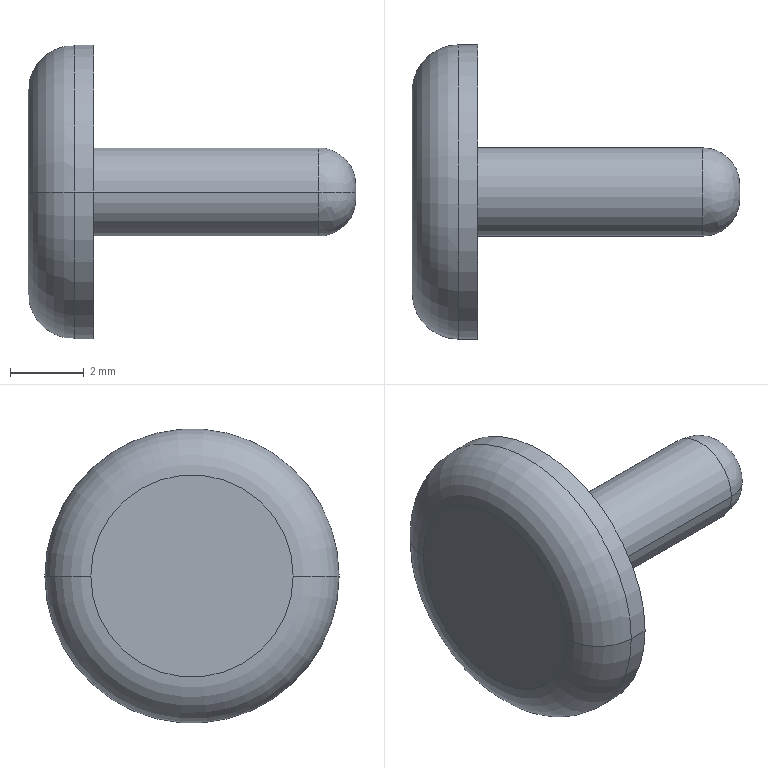Part | STEP file | SR_4060B_1 | 1 solid | 14 faces | box 8.9 x 8 x 8 mm | volume 92.138 mm3 | plane 4 | cylinder 4 | spline 2 | cone 2 | torus 2 | commonest cylinder face diameters 2.4 x2 8 x2
STEP:
#1=CARTESIAN_POINT('',(0.,0.,0.));
#2=DIRECTION('',(0.,0.,1.));
#3=DIRECTION('',(1.,0.,0.));
#4=AXIS2_PLACEMENT_3D('',#1,#2,#3);
#5=CARTESIAN_POINT('',(8.9,0.2,0.));
#6=VERTEX_POINT('',#5);
#7=CARTESIAN_POINT('',(8.9,-0.2,0.));
#8=VERTEX_POINT('',#7);
#9=CARTESIAN_POINT('',(8.9,0.,0.));
#10=DIRECTION('',(-1.,0.,0.));
#11=DIRECTION('',(0.,1.,0.));
#12=AXIS2_PLACEMENT_3D('',#9,#10,#11);
#13=CIRCLE('',#12,0.2);
#14=CARTESIAN_POINT('',(8.9,0.,0.));
#15=DIRECTION('',(1.,0.,0.));
#16=DIRECTION('',(0.,-1.,0.));
#17=AXIS2_PLACEMENT_3D('',#14,#15,#16);
#18=PLANE('',#17);
#19=CARTESIAN_POINT('',(-0.2,0.));
#20=CARTESIAN_POINT('',(-0.2,0.3464));
#21=CARTESIAN_POINT('',(0.1,0.1732));
#22=CARTESIAN_POINT('',(0.4,0.));
#23=CARTESIAN_POINT('',(0.1,-0.1732));
#24=CARTESIAN_POINT('',(-0.2,-0.3464));
#25=CARTESIAN_POINT('',(-0.2,0.));
#26=(BOUNDED_CURVE()B_SPLINE_CURVE(2,(#19,#20,#21,#22,#23,#24,#25),.UNSPECIFIED.,.T.,.F.)B_SPLINE_CURVE_WITH_KNOTS((1,2,2,2,2,1),(-2.094,0.,2.094,4.189,6.283,8.378),.UNSPECIFIED.)CURVE()GEOMETRIC_REPRESENTATION_ITEM()RATIONAL_B_SPLINE_CURVE((1.,0.5,1.,0.5,1.,0.5,1.))REPRESENTATION_ITEM(''));
#27=(GEOMETRIC_REPRESENTATION_CONTEXT(2)PARAMETRIC_REPRESENTATION_CONTEXT()REPRESENTATION_CONTEXT('',''));
#28=DEFINITIONAL_REPRESENTATION('',(#26),#27);
#29=PCURVE('',#18,#28);
#30=CARTESIAN_POINT('',(7.869,-1.195,0.1035));
#31=CARTESIAN_POINT('',(8.484,-1.214,0.1052));
#32=CARTESIAN_POINT('',(8.919,-0.7808,0.06762));
#33=CARTESIAN_POINT('',(8.9,-0.168,0.01455));
#34=CARTESIAN_POINT('',(7.869,-1.26,-0.6455));
#35=CARTESIAN_POINT('',(8.484,-1.28,-0.6559));
#36=CARTESIAN_POINT('',(8.919,-0.8231,-0.4217));
#37=CARTESIAN_POINT('',(8.9,-0.1771,-0.09072));
#38=CARTESIAN_POINT('',(7.869,-0.7518,-1.2));
#39=CARTESIAN_POINT('',(8.484,-0.7639,-1.219));
#40=CARTESIAN_POINT('',(8.919,-0.4912,-0.7837));
#41=CARTESIAN_POINT('',(8.9,-0.1057,-0.1686));
#42=CARTESIAN_POINT('',(7.869,0.,-1.2));
#43=CARTESIAN_POINT('',(8.484,0.,-1.219));
#44=CARTESIAN_POINT('',(8.919,0.,-0.7837));
#45=CARTESIAN_POINT('',(8.9,0.,-0.1686));
#46=CARTESIAN_POINT('',(7.869,0.7518,-1.2));
#47=CARTESIAN_POINT('',(8.484,0.7639,-1.219));
#48=CARTESIAN_POINT('',(8.919,0.4912,-0.7837));
#49=CARTESIAN_POINT('',(8.9,0.1057,-0.1686));
#50=CARTESIAN_POINT('',(7.869,1.26,-0.6455));
#51=CARTESIAN_POINT('',(8.484,1.28,-0.6559));
#52=CARTESIAN_POINT('',(8.919,0.8231,-0.4217));
#53=CARTESIAN_POINT('',(8.9,0.1771,-0.09072));
#54=CARTESIAN_POINT('',(7.869,1.195,0.1035));
#55=CARTESIAN_POINT('',(8.484,1.214,0.1052));
#56=CARTESIAN_POINT('',(8.919,0.7808,0.06762));
#57=CARTESIAN_POINT('',(8.9,0.168,0.01455));
#58=(BOUNDED_SURFACE()B_SPLINE_SURFACE(3,3,((#30,#31,#32,#33),(#34,#35,#36,#37),(#38,#39,#40,#41),(#42,#43,#44,#45),(#46,#47,#48,#49),(#50,#51,#52,#53),(#54,#55,#56,#57)),.UNSPECIFIED.,.F.,.F.,.F.)B_SPLINE_SURFACE_WITH_KNOTS((4,3,4),(4,4),(0.,1.,2.),(0.,1.),.PIECEWISE_BEZIER_KNOTS.)GEOMETRIC_REPRESENTATION_ITEM()RATIONAL_B_SPLINE_SURFACE(((1.417,1.119,1.119,1.417),(1.111,0.8771,0.8771,1.111),(1.111,0.8771,0.8771,1.111),(1.417,1.119,1.119,1.417),(1.111,0.8771,0.8771,1.111),(1.111,0.8771,0.8771,1.111),(1.417,1.119,1.119,1.417)))REPRESENTATION_ITEM('')SURFACE());
#59=CARTESIAN_POINT('',(1.942,0.9786));
#60=CARTESIAN_POINT('',(1.911,0.9786));
#61=CARTESIAN_POINT('',(1.851,0.9786));
#62=CARTESIAN_POINT('',(1.764,0.9786));
#63=CARTESIAN_POINT('',(1.68,0.9786));
#64=CARTESIAN_POINT('',(1.597,0.9786));
#65=CARTESIAN_POINT('',(1.516,0.9786));
#66=CARTESIAN_POINT('',(1.435,0.9786));
#67=CARTESIAN_POINT('',(1.353,0.9786));
#68=CARTESIAN_POINT('',(1.27,0.9786));
#69=CARTESIAN_POINT('',(1.184,0.9786));
#70=CARTESIAN_POINT('',(1.095,0.9786));
#71=CARTESIAN_POINT('',(1.,0.9786));
#72=CARTESIAN_POINT('',(0.9049,0.9786));
#73=CARTESIAN_POINT('',(0.816,0.9786));
#74=CARTESIAN_POINT('',(0.7302,0.9786));
#75=CARTESIAN_POINT('',(0.6469,0.9786));
#76=CARTESIAN_POINT('',(0.5651,0.9786));
#77=CARTESIAN_POINT('',(0.484,0.9786));
#78=CARTESIAN_POINT('',(0.4027,0.9786));
#79=CARTESIAN_POINT('',(0.3204,0.9786));
#80=CARTESIAN_POINT('',(0.2363,0.9786));
#81=CARTESIAN_POINT('',(0.1493,0.9786));
#82=CARTESIAN_POINT('',(0.0887,0.9786));
#83=CARTESIAN_POINT('',(0.05755,0.9786));
#84=B_SPLINE_CURVE_WITH_KNOTS('',3,(#59,#60,#61,#62,#63,#64,#65,#66,#67,#68,#69,#70,#71,#72,#73,#74,#75,#76,#77,#78,#79,#80,#81,#82,#83),.UNSPECIFIED.,.F.,.F.,(4,1,1,1,1,1,1,1,1,1,1,1,1,1,1,1,1,1,1,1,1,1,4),(0.,0.1428,0.2856,0.4284,0.5712,0.714,0.8568,0.9996,1.142,1.285,1.428,1.571,1.714,1.856,1.999,2.142,2.285,2.428,2.57,2.713,2.856,2.999,3.142),.QUASI_UNIFORM_KNOTS.);
#85=(GEOMETRIC_REPRESENTATION_CONTEXT(2)PARAMETRIC_REPRESENTATION_CONTEXT()REPRESENTATION_CONTEXT('',''));
#86=DEFINITIONAL_REPRESENTATION('',(#84),#85);
#87=PCURVE('',#58,#86);
#88=SURFACE_CURVE('',#13,(#29,#87),.PCURVE_S1.);
#89=EDGE_CURVE('',#6,#8,#88,.T.);
#90=ORIENTED_EDGE('',*,*,#89,.T.);
#91=CARTESIAN_POINT('',(8.9,0.,0.));
#92=DIRECTION('',(1.,0.,0.));
#93=DIRECTION('',(0.,1.,0.));
#94=AXIS2_PLACEMENT_3D('',#91,#92,#93);
#95=CIRCLE('',#94,0.2);
#96=CARTESIAN_POINT('',(0.,0.));
#97=DIRECTION('',(-1.,0.));
#98=AXIS2_PLACEMENT_2D('',#96,#97);
#99=CIRCLE('',#98,0.2);
#100=(GEOMETRIC_REPRESENTATION_CONTEXT(2)PARAMETRIC_REPRESENTATION_CONTEXT()REPRESENTATION_CONTEXT('',''));
#101=DEFINITIONAL_REPRESENTATION('',(#99),#100);
#102=PCURVE('',#18,#101);
#103=CARTESIAN_POINT('',(7.869,1.195,-0.1035));
#104=CARTESIAN_POINT('',(8.484,1.214,-0.1052));
#105=CARTESIAN_POINT('',(8.919,0.7808,-0.06762));
#106=CARTESIAN_POINT('',(8.9,0.168,-0.01455));
#107=CARTESIAN_POINT('',(7.869,1.26,0.6455));
#108=CARTESIAN_POINT('',(8.484,1.28,0.6559));
#109=CARTESIAN_POINT('',(8.919,0.8231,0.4217));
#110=CARTESIAN_POINT('',(8.9,0.1771,0.09072));
#111=CARTESIAN_POINT('',(7.869,0.7518,1.2));
#112=CARTESIAN_POINT('',(8.484,0.7639,1.219));
#113=CARTESIAN_POINT('',(8.919,0.4912,0.7837));
#114=CARTESIAN_POINT('',(8.9,0.1057,0.1686));
#115=CARTESIAN_POINT('',(7.869,0.,1.2));
#116=CARTESIAN_POINT('',(8.484,0.,1.219));
#117=CARTESIAN_POINT('',(8.919,0.,0.7837));
#118=CARTESIAN_POINT('',(8.9,0.,0.1686));
#119=CARTESIAN_POINT('',(7.869,-0.7518,1.2));
#120=CARTESIAN_POINT('',(8.484,-0.7639,1.219));
#121=CARTESIAN_POINT('',(8.919,-0.4912,0.7837));
#122=CARTESIAN_POINT('',(8.9,-0.1057,0.1686));
#123=CARTESIAN_POINT('',(7.869,-1.26,0.6455));
#124=CARTESIAN_POINT('',(8.484,-1.28,0.6559));
#125=CARTESIAN_POINT('',(8.919,-0.8231,0.4217));
#126=CARTESIAN_POINT('',(8.9,-0.1771,0.09072));
#127=CARTESIAN_POINT('',(7.869,-1.195,-0.1035));
#128=CARTESIAN_POINT('',(8.484,-1.214,-0.1052));
#129=CARTESIAN_POINT('',(8.919,-0.7808,-0.06762));
#130=CARTESIAN_POINT('',(8.9,-0.168,-0.01455));
#131=(BOUNDED_SURFACE()B_SPLINE_SURFACE(3,3,((#103,#104,#105,#106),(#107,#108,#109,#110),(#111,#112,#113,#114),(#115,#116,#117,#118),(#119,#120,#121,#122),(#123,#124,#125,#126),(#127,#128,#129,#130)),.UNSPECIFIED.,.F.,.F.,.F.)B_SPLINE_SURFACE_WITH_KNOTS((4,3,4),(4,4),(0.,1.,2.),(0.,1.),.PIECEWISE_BEZIER_KNOTS.)GEOMETRIC_REPRESENTATION_ITEM()RATIONAL_B_SPLINE_SURFACE(((1.417,1.119,1.119,1.417),(1.111,0.8771,0.8771,1.111),(1.111,0.8771,0.8771,1.111),(1.417,1.119,1.119,1.417),(1.111,0.8771,0.8771,1.111),(1.111,0.8771,0.8771,1.111),(1.417,1.119,1.119,1.417)))REPRESENTATION_ITEM('')SURFACE());
#132=CARTESIAN_POINT('',(0.05755,0.9786));
#133=CARTESIAN_POINT('',(0.0887,0.9786));
#134=CARTESIAN_POINT('',(0.1493,0.9786));
#135=CARTESIAN_POINT('',(0.2363,0.9786));
#136=CARTESIAN_POINT('',(0.3204,0.9786));
#137=CARTESIAN_POINT('',(0.4027,0.9786));
#138=CARTESIAN_POINT('',(0.484,0.9786));
#139=CARTESIAN_POINT('',(0.5651,0.9786));
#140=CARTESIAN_POINT('',(0.6469,0.9786));
#141=CARTESIAN_POINT('',(0.7302,0.9786));
#142=CARTESIAN_POINT('',(0.816,0.9786));
#143=CARTESIAN_POINT('',(0.9049,0.9786));
#144=CARTESIAN_POINT('',(1.,0.9786));
#145=CARTESIAN_POINT('',(1.095,0.9786));
#146=CARTESIAN_POINT('',(1.184,0.9786));
#147=CARTESIAN_POINT('',(1.27,0.9786));
#148=CARTESIAN_POINT('',(1.353,0.9786));
#149=CARTESIAN_POINT('',(1.435,0.9786));
#150=CARTESIAN_POINT('',(1.516,0.9786));
#151=CARTESIAN_POINT('',(1.597,0.9786));
#152=CARTESIAN_POINT('',(1.68,0.9786));
#153=CARTESIAN_POINT('',(1.764,0.9786));
#154=CARTESIAN_POINT('',(1.851,0.9786));
#155=CARTESIAN_POINT('',(1.911,0.9786));
#156=CARTESIAN_POINT('',(1.942,0.9786));
#157=B_SPLINE_CURVE_WITH_KNOTS('',3,(#132,#133,#134,#135,#136,#137,#138,#139,#140,#141,#142,#143,#144,#145,#146,#147,#148,#149,#150,#151,#152,#153,#154,#155,#156),.UNSPECIFIED.,.F.,.F.,(4,1,1,1,1,1,1,1,1,1,1,1,1,1,1,1,1,1,1,1,1,1,4),(0.,0.1428,0.2856,0.4284,0.5712,0.714,0.8568,0.9996,1.142,1.285,1.428,1.571,1.714,1.856,1.999,2.142,2.285,2.428,2.57,2.713,2.856,2.999,3.142),.QUASI_UNIFORM_KNOTS.);
#158=(GEOMETRIC_REPRESENTATION_CONTEXT(2)PARAMETRIC_REPRESENTATION_CONTEXT()REPRESENTATION_CONTEXT('',''));
#159=DEFINITIONAL_REPRESENTATION('',(#157),#158);
#160=PCURVE('',#131,#159);
#161=SURFACE_CURVE('',#95,(#102,#160),.PCURVE_S1.);
#162=EDGE_CURVE('',#6,#8,#161,.T.);
#163=ORIENTED_EDGE('',*,*,#162,.F.);
#164=EDGE_LOOP('',(#90,#163));
#165=FACE_BOUND('',#164,.F.);
#166=ADVANCED_FACE('',(#165),#18,.T.);
#167=ORIENTED_EDGE('',*,*,#89,.T.);
#168=CARTESIAN_POINT('',(7.9,-1.2,0.));
#169=VERTEX_POINT('',#168);
#170=CARTESIAN_POINT('',(7.9,-0.2,0.));
#171=DIRECTION('',(0.,0.,-1.));
#172=DIRECTION('',(1.,0.,0.));
#173=AXIS2_PLACEMENT_3D('',#170,#171,#172);
#174=CIRCLE('',#173,1.);
#175=CARTESIAN_POINT('',(0.05755,0.9786));
#176=CARTESIAN_POINT('',(0.05755,0.9625));
#177=CARTESIAN_POINT('',(0.05755,0.9307));
#178=CARTESIAN_POINT('',(0.05755,0.8844));
#179=CARTESIAN_POINT('',(0.05755,0.8391));
#180=CARTESIAN_POINT('',(0.05755,0.7948));
#181=CARTESIAN_POINT('',(0.05755,0.7512));
#182=CARTESIAN_POINT('',(0.05755,0.7084));
#183=CARTESIAN_POINT('',(0.05755,0.6661));
#184=CARTESIAN_POINT('',(0.05755,0.6242));
#185=CARTESIAN_POINT('',(0.05755,0.5826));
#186=CARTESIAN_POINT('',(0.05755,0.5412));
#187=CARTESIAN_POINT('',(0.05755,0.5));
#188=CARTESIAN_POINT('',(0.05755,0.4588));
#189=CARTESIAN_POINT('',(0.05755,0.4174));
#190=CARTESIAN_POINT('',(0.05755,0.3758));
#191=CARTESIAN_POINT('',(0.05755,0.3339));
#192=CARTESIAN_POINT('',(0.05755,0.2916));
#193=CARTESIAN_POINT('',(0.05755,0.2488));
#194=CARTESIAN_POINT('',(0.05755,0.2052));
#195=CARTESIAN_POINT('',(0.05755,0.1609));
#196=CARTESIAN_POINT('',(0.05755,0.1156));
#197=CARTESIAN_POINT('',(0.05755,0.06926));
#198=CARTESIAN_POINT('',(0.05755,0.03751));
#199=CARTESIAN_POINT('',(0.05755,0.0214));
#200=B_SPLINE_CURVE_WITH_KNOTS('',3,(#175,#176,#177,#178,#179,#180,#181,#182,#183,#184,#185,#186,#187,#188,#189,#190,#191,#192,#193,#194,#195,#196,#197,#198,#199),.UNSPECIFIED.,.F.,.F.,(4,1,1,1,1,1,1,1,1,1,1,1,1,1,1,1,1,1,1,1,1,1,4),(0.,0.0714,0.1428,0.2142,0.2856,0.357,0.4284,0.4998,0.5712,0.6426,0.714,0.7854,0.8568,0.9282,0.9996,1.071,1.142,1.214,1.285,1.357,1.428,1.499,1.571),.QUASI_UNIFORM_KNOTS.);
#201=(GEOMETRIC_REPRESENTATION_CONTEXT(2)PARAMETRIC_REPRESENTATION_CONTEXT()REPRESENTATION_CONTEXT('',''));
#202=DEFINITIONAL_REPRESENTATION('',(#200),#201);
#203=PCURVE('',#58,#202);
#204=CARTESIAN_POINT('',(1.942,0.9786));
#205=CARTESIAN_POINT('',(1.942,0.9625));
#206=CARTESIAN_POINT('',(1.942,0.9307));
#207=CARTESIAN_POINT('',(1.942,0.8844));
#208=CARTESIAN_POINT('',(1.942,0.8391));
#209=CARTESIAN_POINT('',(1.942,0.7948));
#210=CARTESIAN_POINT('',(1.942,0.7512));
#211=CARTESIAN_POINT('',(1.942,0.7084));
#212=CARTESIAN_POINT('',(1.942,0.6661));
#213=CARTESIAN_POINT('',(1.942,0.6242));
#214=CARTESIAN_POINT('',(1.942,0.5826));
#215=CARTESIAN_POINT('',(1.942,0.5412));
#216=CARTESIAN_POINT('',(1.942,0.5));
#217=CARTESIAN_POINT('',(1.942,0.4588));
#218=CARTESIAN_POINT('',(1.942,0.4174));
#219=CARTESIAN_POINT('',(1.942,0.3758));
#220=CARTESIAN_POINT('',(1.942,0.3339));
#221=CARTESIAN_POINT('',(1.942,0.2916));
#222=CARTESIAN_POINT('',(1.942,0.2488));
#223=CARTESIAN_POINT('',(1.942,0.2052));
#224=CARTESIAN_POINT('',(1.942,0.1609));
#225=CARTESIAN_POINT('',(1.942,0.1156));
#226=CARTESIAN_POINT('',(1.942,0.06926));
#227=CARTESIAN_POINT('',(1.942,0.03751));
#228=CARTESIAN_POINT('',(1.942,0.0214));
#229=B_SPLINE_CURVE_WITH_KNOTS('',3,(#204,#205,#206,#207,#208,#209,#210,#211,#212,#213,#214,#215,#216,#217,#218,#219,#220,#221,#222,#223,#224,#225,#226,#227,#228),.UNSPECIFIED.,.F.,.F.,(4,1,1,1,1,1,1,1,1,1,1,1,1,1,1,1,1,1,1,1,1,1,4),(0.,0.0714,0.1428,0.2142,0.2856,0.357,0.4284,0.4998,0.5712,0.6426,0.714,0.7854,0.8568,0.9282,0.9996,1.071,1.142,1.214,1.285,1.357,1.428,1.499,1.571),.QUASI_UNIFORM_KNOTS.);
#230=(GEOMETRIC_REPRESENTATION_CONTEXT(2)PARAMETRIC_REPRESENTATION_CONTEXT()REPRESENTATION_CONTEXT('',''));
#231=DEFINITIONAL_REPRESENTATION('',(#229),#230);
#232=PCURVE('',#131,#231);
#233=SURFACE_CURVE('',#174,(#203,#232),.PCURVE_S1.);
#234=EDGE_CURVE('',#8,#169,#233,.T.);
#235=ORIENTED_EDGE('',*,*,#234,.T.);
#236=CARTESIAN_POINT('',(7.9,1.2,0.));
#237=VERTEX_POINT('',#236);
#238=CARTESIAN_POINT('',(7.9,0.,0.));
#239=DIRECTION('',(-1.,0.,0.));
#240=DIRECTION('',(0.,1.,0.));
#241=AXIS2_PLACEMENT_3D('',#238,#239,#240);
#242=CIRCLE('',#241,1.2);
#243=CARTESIAN_POINT('',(1.942,0.0214));
#244=CARTESIAN_POINT('',(1.911,0.0214));
#245=CARTESIAN_POINT('',(1.851,0.0214));
#246=CARTESIAN_POINT('',(1.764,0.0214));
#247=CARTESIAN_POINT('',(1.68,0.0214));
#248=CARTESIAN_POINT('',(1.597,0.0214));
#249=CARTESIAN_POINT('',(1.516,0.0214));
#250=CARTESIAN_POINT('',(1.435,0.0214));
#251=CARTESIAN_POINT('',(1.353,0.0214));
#252=CARTESIAN_POINT('',(1.27,0.0214));
#253=CARTESIAN_POINT('',(1.184,0.0214));
#254=CARTESIAN_POINT('',(1.095,0.0214));
#255=CARTESIAN_POINT('',(1.,0.0214));
#256=CARTESIAN_POINT('',(0.9049,0.0214));
#257=CARTESIAN_POINT('',(0.816,0.0214));
#258=CARTESIAN_POINT('',(0.7302,0.0214));
#259=CARTESIAN_POINT('',(0.6469,0.0214));
#260=CARTESIAN_POINT('',(0.5651,0.0214));
#261=CARTESIAN_POINT('',(0.484,0.0214));
#262=CARTESIAN_POINT('',(0.4027,0.0214));
#263=CARTESIAN_POINT('',(0.3204,0.0214));
#264=CARTESIAN_POINT('',(0.2363,0.0214));
#265=CARTESIAN_POINT('',(0.1493,0.0214));
#266=CARTESIAN_POINT('',(0.0887,0.0214));
#267=CARTESIAN_POINT('',(0.05755,0.0214));
#268=B_SPLINE_CURVE_WITH_KNOTS('',3,(#243,#244,#245,#246,#247,#248,#249,#250,#251,#252,#253,#254,#255,#256,#257,#258,#259,#260,#261,#262,#263,#264,#265,#266,#267),.UNSPECIFIED.,.F.,.F.,(4,1,1,1,1,1,1,1,1,1,1,1,1,1,1,1,1,1,1,1,1,1,4),(0.,0.1428,0.2856,0.4284,0.5712,0.714,0.8568,0.9996,1.142,1.285,1.428,1.571,1.714,1.856,1.999,2.142,2.285,2.428,2.57,2.713,2.856,2.999,3.142),.QUASI_UNIFORM_KNOTS.);
#269=(GEOMETRIC_REPRESENTATION_CONTEXT(2)PARAMETRIC_REPRESENTATION_CONTEXT()REPRESENTATION_CONTEXT('',''));
#270=DEFINITIONAL_REPRESENTATION('',(#268),#269);
#271=PCURVE('',#58,#270);
#272=CARTESIAN_POINT('',(-0.445,0.,0.));
#273=DIRECTION('',(1.,0.,0.));
#274=DIRECTION('',(0.,-1.,0.));
#275=AXIS2_PLACEMENT_3D('',#272,#273,#274);
#276=CYLINDRICAL_SURFACE('',#275,1.2);
#277=CARTESIAN_POINT('',(3.142,8.345));
#278=DIRECTION('',(-1.,0.));
#279=VECTOR('',#278,1.);
#280=LINE('',#277,#279);
#281=(GEOMETRIC_REPRESENTATION_CONTEXT(2)PARAMETRIC_REPRESENTATION_CONTEXT()REPRESENTATION_CONTEXT('',''));
#282=DEFINITIONAL_REPRESENTATION('',(#280),#281);
#283=PCURVE('',#276,#282);
#284=SURFACE_CURVE('',#242,(#271,#283),.PCURVE_S1.);
#285=EDGE_CURVE('',#237,#169,#284,.T.);
#286=ORIENTED_EDGE('',*,*,#285,.F.);
#287=CARTESIAN_POINT('',(7.9,0.2,0.));
#288=DIRECTION('',(0.,0.,1.));
#289=DIRECTION('',(1.,0.,0.));
#290=AXIS2_PLACEMENT_3D('',#287,#288,#289);
#291=CIRCLE('',#290,1.);
#292=CARTESIAN_POINT('',(1.942,0.9786));
#293=CARTESIAN_POINT('',(1.942,0.9625));
#294=CARTESIAN_POINT('',(1.942,0.9307));
#295=CARTESIAN_POINT('',(1.942,0.8844));
#296=CARTESIAN_POINT('',(1.942,0.8391));
#297=CARTESIAN_POINT('',(1.942,0.7948));
#298=CARTESIAN_POINT('',(1.942,0.7512));
#299=CARTESIAN_POINT('',(1.942,0.7084));
#300=CARTESIAN_POINT('',(1.942,0.6661));
#301=CARTESIAN_POINT('',(1.942,0.6242));
#302=CARTESIAN_POINT('',(1.942,0.5826));
#303=CARTESIAN_POINT('',(1.942,0.5412));
#304=CARTESIAN_POINT('',(1.942,0.5));
#305=CARTESIAN_POINT('',(1.942,0.4588));
#306=CARTESIAN_POINT('',(1.942,0.4174));
#307=CARTESIAN_POINT('',(1.942,0.3758));
#308=CARTESIAN_POINT('',(1.942,0.3339));
#309=CARTESIAN_POINT('',(1.942,0.2916));
#310=CARTESIAN_POINT('',(1.942,0.2488));
#311=CARTESIAN_POINT('',(1.942,0.2052));
#312=CARTESIAN_POINT('',(1.942,0.1609));
#313=CARTESIAN_POINT('',(1.942,0.1156));
#314=CARTESIAN_POINT('',(1.942,0.06926));
#315=CARTESIAN_POINT('',(1.942,0.03751));
#316=CARTESIAN_POINT('',(1.942,0.0214));
#317=B_SPLINE_CURVE_WITH_KNOTS('',3,(#292,#293,#294,#295,#296,#297,#298,#299,#300,#301,#302,#303,#304,#305,#306,#307,#308,#309,#310,#311,#312,#313,#314,#315,#316),.UNSPECIFIED.,.F.,.F.,(4,1,1,1,1,1,1,1,1,1,1,1,1,1,1,1,1,1,1,1,1,1,4),(0.,0.0714,0.1428,0.2142,0.2856,0.357,0.4284,0.4998,0.5712,0.6426,0.714,0.7854,0.8568,0.9282,0.9996,1.071,1.142,1.214,1.285,1.357,1.428,1.499,1.571),.QUASI_UNIFORM_KNOTS.);
#318=(GEOMETRIC_REPRESENTATION_CONTEXT(2)PARAMETRIC_REPRESENTATION_CONTEXT()REPRESENTATION_CONTEXT('',''));
#319=DEFINITIONAL_REPRESENTATION('',(#317),#318);
#320=PCURVE('',#58,#319);
#321=CARTESIAN_POINT('',(0.05755,0.9786));
#322=CARTESIAN_POINT('',(0.05755,0.9625));
#323=CARTESIAN_POINT('',(0.05755,0.9307));
#324=CARTESIAN_POINT('',(0.05755,0.8844));
#325=CARTESIAN_POINT('',(0.05755,0.8391));
#326=CARTESIAN_POINT('',(0.05755,0.7948));
#327=CARTESIAN_POINT('',(0.05755,0.7512));
#328=CARTESIAN_POINT('',(0.05755,0.7084));
#329=CARTESIAN_POINT('',(0.05755,0.6661));
#330=CARTESIAN_POINT('',(0.05755,0.6242));
#331=CARTESIAN_POINT('',(0.05755,0.5826));
#332=CARTESIAN_POINT('',(0.05755,0.5412));
#333=CARTESIAN_POINT('',(0.05755,0.5));
#334=CARTESIAN_POINT('',(0.05755,0.4588));
#335=CARTESIAN_POINT('',(0.05755,0.4174));
#336=CARTESIAN_POINT('',(0.05755,0.3758));
#337=CARTESIAN_POINT('',(0.05755,0.3339));
#338=CARTESIAN_POINT('',(0.05755,0.2916));
#339=CARTESIAN_POINT('',(0.05755,0.2488));
#340=CARTESIAN_POINT('',(0.05755,0.2052));
#341=CARTESIAN_POINT('',(0.05755,0.1609));
#342=CARTESIAN_POINT('',(0.05755,0.1156));
#343=CARTESIAN_POINT('',(0.05755,0.06926));
#344=CARTESIAN_POINT('',(0.05755,0.03751));
#345=CARTESIAN_POINT('',(0.05755,0.0214));
#346=B_SPLINE_CURVE_WITH_KNOTS('',3,(#321,#322,#323,#324,#325,#326,#327,#328,#329,#330,#331,#332,#333,#334,#335,#336,#337,#338,#339,#340,#341,#342,#343,#344,#345),.UNSPECIFIED.,.F.,.F.,(4,1,1,1,1,1,1,1,1,1,1,1,1,1,1,1,1,1,1,1,1,1,4),(0.,0.0714,0.1428,0.2142,0.2856,0.357,0.4284,0.4998,0.5712,0.6426,0.714,0.7854,0.8568,0.9282,0.9996,1.071,1.142,1.214,1.285,1.357,1.428,1.499,1.571),.QUASI_UNIFORM_KNOTS.);
#347=(GEOMETRIC_REPRESENTATION_CONTEXT(2)PARAMETRIC_REPRESENTATION_CONTEXT()REPRESENTATION_CONTEXT('',''));
#348=DEFINITIONAL_REPRESENTATION('',(#346),#347);
#349=PCURVE('',#131,#348);
#350=SURFACE_CURVE('',#291,(#320,#349),.PCURVE_S1.);
#351=EDGE_CURVE('',#6,#237,#350,.T.);
#352=ORIENTED_EDGE('',*,*,#351,.F.);
#353=EDGE_LOOP('',(#167,#235,#286,#352));
#354=FACE_BOUND('',#353,.T.);
#355=ADVANCED_FACE('',(#354),#58,.T.);
#356=CARTESIAN_POINT('',(7.9,0.,0.));
#357=DIRECTION('',(1.,0.,0.));
#358=DIRECTION('',(0.,1.,0.));
#359=AXIS2_PLACEMENT_3D('',#356,#357,#358);
#360=CIRCLE('',#359,1.2);
#361=CARTESIAN_POINT('',(0.05755,0.0214));
#362=CARTESIAN_POINT('',(0.0887,0.0214));
#363=CARTESIAN_POINT('',(0.1493,0.0214));
#364=CARTESIAN_POINT('',(0.2363,0.0214));
#365=CARTESIAN_POINT('',(0.3204,0.0214));
#366=CARTESIAN_POINT('',(0.4027,0.0214));
#367=CARTESIAN_POINT('',(0.484,0.0214));
#368=CARTESIAN_POINT('',(0.5651,0.0214));
#369=CARTESIAN_POINT('',(0.6469,0.0214));
#370=CARTESIAN_POINT('',(0.7302,0.0214));
#371=CARTESIAN_POINT('',(0.816,0.0214));
#372=CARTESIAN_POINT('',(0.9049,0.0214));
#373=CARTESIAN_POINT('',(1.,0.0214));
#374=CARTESIAN_POINT('',(1.095,0.0214));
#375=CARTESIAN_POINT('',(1.184,0.0214));
#376=CARTESIAN_POINT('',(1.27,0.0214));
#377=CARTESIAN_POINT('',(1.353,0.0214));
#378=CARTESIAN_POINT('',(1.435,0.0214));
#379=CARTESIAN_POINT('',(1.516,0.0214));
#380=CARTESIAN_POINT('',(1.597,0.0214));
#381=CARTESIAN_POINT('',(1.68,0.0214));
#382=CARTESIAN_POINT('',(1.764,0.0214));
#383=CARTESIAN_POINT('',(1.851,0.0214));
#384=CARTESIAN_POINT('',(1.911,0.0214));
#385=CARTESIAN_POINT('',(1.942,0.0214));
#386=B_SPLINE_CURVE_WITH_KNOTS('',3,(#361,#362,#363,#364,#365,#366,#367,#368,#369,#370,#371,#372,#373,#374,#375,#376,#377,#378,#379,#380,#381,#382,#383,#384,#385),.UNSPECIFIED.,.F.,.F.,(4,1,1,1,1,1,1,1,1,1,1,1,1,1,1,1,1,1,1,1,1,1,4),(0.,0.1428,0.2856,0.4284,0.5712,0.714,0.8568,0.9996,1.142,1.285,1.428,1.571,1.714,1.856,1.999,2.142,2.285,2.428,2.57,2.713,2.856,2.999,3.142),.QUASI_UNIFORM_KNOTS.);
#387=(GEOMETRIC_REPRESENTATION_CONTEXT(2)PARAMETRIC_REPRESENTATION_CONTEXT()REPRESENTATION_CONTEXT('',''));
#388=DEFINITIONAL_REPRESENTATION('',(#386),#387);
#389=PCURVE('',#131,#388);
#390=CARTESIAN_POINT('',(-0.445,0.,0.));
#391=DIRECTION('',(1.,0.,0.));
#392=DIRECTION('',(0.,-1.,0.));
#393=AXIS2_PLACEMENT_3D('',#390,#391,#392);
#394=CYLINDRICAL_SURFACE('',#393,1.2);
#395=CARTESIAN_POINT('',(3.142,8.345));
#396=DIRECTION('',(1.,0.));
#397=VECTOR('',#396,1.);
#398=LINE('',#395,#397);
#399=(GEOMETRIC_REPRESENTATION_CONTEXT(2)PARAMETRIC_REPRESENTATION_CONTEXT()REPRESENTATION_CONTEXT('',''));
#400=DEFINITIONAL_REPRESENTATION('',(#398),#399);
#401=PCURVE('',#394,#400);
#402=SURFACE_CURVE('',#360,(#389,#401),.PCURVE_S1.);
#403=EDGE_CURVE('',#237,#169,#402,.T.);
#404=ORIENTED_EDGE('',*,*,#403,.T.);
#405=ORIENTED_EDGE('',*,*,#234,.F.);
#406=ORIENTED_EDGE('',*,*,#162,.F.);
#407=ORIENTED_EDGE('',*,*,#351,.T.);
#408=EDGE_LOOP('',(#404,#405,#406,#407));
#409=FACE_BOUND('',#408,.T.);
#410=ADVANCED_FACE('',(#409),#131,.T.);
#411=CARTESIAN_POINT('',(0.9,1.2,0.));
#412=VERTEX_POINT('',#411);
#413=CARTESIAN_POINT('',(0.9,-1.2,0.));
#414=VERTEX_POINT('',#413);
#415=CARTESIAN_POINT('',(0.9,0.,0.));
#416=DIRECTION('',(1.,0.,0.));
#417=DIRECTION('',(0.,1.,0.));
#418=AXIS2_PLACEMENT_3D('',#415,#416,#417);
#419=CIRCLE('',#418,1.2);
#420=CARTESIAN_POINT('',(3.142,1.345));
#421=DIRECTION('',(1.,0.));
#422=VECTOR('',#421,1.);
#423=LINE('',#420,#422);
#424=(GEOMETRIC_REPRESENTATION_CONTEXT(2)PARAMETRIC_REPRESENTATION_CONTEXT()REPRESENTATION_CONTEXT('',''));
#425=DEFINITIONAL_REPRESENTATION('',(#423),#424);
#426=PCURVE('',#394,#425);
#427=CARTESIAN_POINT('',(0.9,0.,0.));
#428=DIRECTION('',(1.,0.,0.));
#429=DIRECTION('',(0.,-1.,0.));
#430=AXIS2_PLACEMENT_3D('',#427,#428,#429);
#431=PLANE('',#430);
#432=CARTESIAN_POINT('',(0.,0.));
#433=DIRECTION('',(-1.,0.));
#434=AXIS2_PLACEMENT_2D('',#432,#433);
#435=CIRCLE('',#434,1.2);
#436=(GEOMETRIC_REPRESENTATION_CONTEXT(2)PARAMETRIC_REPRESENTATION_CONTEXT()REPRESENTATION_CONTEXT('',''));
#437=DEFINITIONAL_REPRESENTATION('',(#435),#436);
#438=PCURVE('',#431,#437);
#439=SURFACE_CURVE('',#419,(#426,#438),.PCURVE_S1.);
#440=EDGE_CURVE('',#412,#414,#439,.T.);
#441=ORIENTED_EDGE('',*,*,#440,.T.);
#442=CARTESIAN_POINT('',(7.9,-1.2,0.));
#443=DIRECTION('',(-1.,0.,0.));
#444=VECTOR('',#443,1.);
#445=LINE('',#442,#444);
#446=CARTESIAN_POINT('',(6.283,8.345));
#447=DIRECTION('',(0.,-1.));
#448=VECTOR('',#447,1.);
#449=LINE('',#446,#448);
#450=(GEOMETRIC_REPRESENTATION_CONTEXT(2)PARAMETRIC_REPRESENTATION_CONTEXT()REPRESENTATION_CONTEXT('',''));
#451=DEFINITIONAL_REPRESENTATION('',(#449),#450);
#452=PCURVE('',#394,#451);
#453=CARTESIAN_POINT('',(0.,8.345));
#454=DIRECTION('',(0.,-1.));
#455=VECTOR('',#454,1.);
#456=LINE('',#453,#455);
#457=(GEOMETRIC_REPRESENTATION_CONTEXT(2)PARAMETRIC_REPRESENTATION_CONTEXT()REPRESENTATION_CONTEXT('',''));
#458=DEFINITIONAL_REPRESENTATION('',(#456),#457);
#459=PCURVE('',#276,#458);
#460=SURFACE_CURVE('',#445,(#452,#459),.PCURVE_S1.);
#461=EDGE_CURVE('',#169,#414,#460,.T.);
#462=ORIENTED_EDGE('',*,*,#461,.F.);
#463=ORIENTED_EDGE('',*,*,#403,.F.);
#464=CARTESIAN_POINT('',(7.9,1.2,0.));
#465=DIRECTION('',(-1.,0.,0.));
#466=VECTOR('',#465,1.);
#467=LINE('',#464,#466);
#468=CARTESIAN_POINT('',(3.142,8.345));
#469=DIRECTION('',(0.,-1.));
#470=VECTOR('',#469,1.);
#471=LINE('',#468,#470);
#472=(GEOMETRIC_REPRESENTATION_CONTEXT(2)PARAMETRIC_REPRESENTATION_CONTEXT()REPRESENTATION_CONTEXT('',''));
#473=DEFINITIONAL_REPRESENTATION('',(#471),#472);
#474=PCURVE('',#394,#473);
#475=CARTESIAN_POINT('',(3.142,8.345));
#476=DIRECTION('',(0.,-1.));
#477=VECTOR('',#476,1.);
#478=LINE('',#475,#477);
#479=(GEOMETRIC_REPRESENTATION_CONTEXT(2)PARAMETRIC_REPRESENTATION_CONTEXT()REPRESENTATION_CONTEXT('',''));
#480=DEFINITIONAL_REPRESENTATION('',(#478),#479);
#481=PCURVE('',#276,#480);
#482=SURFACE_CURVE('',#467,(#474,#481),.PCURVE_S1.);
#483=EDGE_CURVE('',#237,#412,#482,.T.);
#484=ORIENTED_EDGE('',*,*,#483,.T.);
#485=EDGE_LOOP('',(#441,#462,#463,#484));
#486=FACE_BOUND('',#485,.T.);
#487=ADVANCED_FACE('',(#486),#394,.T.);
#488=ORIENTED_EDGE('',*,*,#285,.T.);
#489=ORIENTED_EDGE('',*,*,#461,.T.);
#490=CARTESIAN_POINT('',(0.9,0.,0.));
#491=DIRECTION('',(-1.,0.,0.));
#492=DIRECTION('',(0.,1.,0.));
#493=AXIS2_PLACEMENT_3D('',#490,#491,#492);
#494=CIRCLE('',#493,1.2);
#495=CARTESIAN_POINT('',(3.142,1.345));
#496=DIRECTION('',(-1.,0.));
#497=VECTOR('',#496,1.);
#498=LINE('',#495,#497);
#499=(GEOMETRIC_REPRESENTATION_CONTEXT(2)PARAMETRIC_REPRESENTATION_CONTEXT()REPRESENTATION_CONTEXT('',''));
#500=DEFINITIONAL_REPRESENTATION('',(#498),#499);
#501=PCURVE('',#276,#500);
#502=CARTESIAN_POINT('',(-1.2,0.));
#503=CARTESIAN_POINT('',(-1.2,2.078));
#504=CARTESIAN_POINT('',(0.6,1.039));
#505=CARTESIAN_POINT('',(2.4,0.));
#506=CARTESIAN_POINT('',(0.6,-1.039));
#507=CARTESIAN_POINT('',(-1.2,-2.078));
#508=CARTESIAN_POINT('',(-1.2,0.));
#509=(BOUNDED_CURVE()B_SPLINE_CURVE(2,(#502,#503,#504,#505,#506,#507,#508),.UNSPECIFIED.,.T.,.F.)B_SPLINE_CURVE_WITH_KNOTS((1,2,2,2,2,1),(-2.094,0.,2.094,4.189,6.283,8.378),.UNSPECIFIED.)CURVE()GEOMETRIC_REPRESENTATION_ITEM()RATIONAL_B_SPLINE_CURVE((1.,0.5,1.,0.5,1.,0.5,1.))REPRESENTATION_ITEM(''));
#510=(GEOMETRIC_REPRESENTATION_CONTEXT(2)PARAMETRIC_REPRESENTATION_CONTEXT()REPRESENTATION_CONTEXT('',''));
#511=DEFINITIONAL_REPRESENTATION('',(#509),#510);
#512=PCURVE('',#431,#511);
#513=SURFACE_CURVE('',#494,(#501,#512),.PCURVE_S1.);
#514=EDGE_CURVE('',#412,#414,#513,.T.);
#515=ORIENTED_EDGE('',*,*,#514,.F.);
#516=ORIENTED_EDGE('',*,*,#483,.F.);
#517=EDGE_LOOP('',(#488,#489,#515,#516));
#518=FACE_BOUND('',#517,.T.);
#519=ADVANCED_FACE('',(#518),#276,.T.);
#520=CARTESIAN_POINT('',(0.9,2.7,0.));
#521=VERTEX_POINT('',#520);
#522=CARTESIAN_POINT('',(0.9,-2.7,0.));
#523=VERTEX_POINT('',#522);
#524=CARTESIAN_POINT('',(0.9,0.,0.));
#525=DIRECTION('',(-1.,0.,0.));
#526=DIRECTION('',(0.,1.,0.));
#527=AXIS2_PLACEMENT_3D('',#524,#525,#526);
#528=CIRCLE('',#527,2.7);
#529=CARTESIAN_POINT('',(-2.7,0.));
#530=CARTESIAN_POINT('',(-2.7,4.677));
#531=CARTESIAN_POINT('',(1.35,2.338));
#532=CARTESIAN_POINT('',(5.4,0.));
#533=CARTESIAN_POINT('',(1.35,-2.338));
#534=CARTESIAN_POINT('',(-2.7,-4.677));
#535=CARTESIAN_POINT('',(-2.7,0.));
#536=(BOUNDED_CURVE()B_SPLINE_CURVE(2,(#529,#530,#531,#532,#533,#534,#535),.UNSPECIFIED.,.T.,.F.)B_SPLINE_CURVE_WITH_KNOTS((1,2,2,2,2,1),(-2.094,0.,2.094,4.189,6.283,8.378),.UNSPECIFIED.)CURVE()GEOMETRIC_REPRESENTATION_ITEM()RATIONAL_B_SPLINE_CURVE((1.,0.5,1.,0.5,1.,0.5,1.))REPRESENTATION_ITEM(''));
#537=(GEOMETRIC_REPRESENTATION_CONTEXT(2)PARAMETRIC_REPRESENTATION_CONTEXT()REPRESENTATION_CONTEXT('',''));
#538=DEFINITIONAL_REPRESENTATION('',(#536),#537);
#539=PCURVE('',#431,#538);
#540=CARTESIAN_POINT('',(1.34,0.,0.));
#541=DIRECTION('',(1.,0.,0.));
#542=DIRECTION('',(0.,-1.,0.));
#543=AXIS2_PLACEMENT_3D('',#540,#541,#542);
#544=CONICAL_SURFACE('',#543,2.965,0.5421);
#545=CARTESIAN_POINT('',(3.142,-0.44));
#546=DIRECTION('',(-1.,0.));
#547=VECTOR('',#546,1.);
#548=LINE('',#545,#547);
#549=(GEOMETRIC_REPRESENTATION_CONTEXT(2)PARAMETRIC_REPRESENTATION_CONTEXT()REPRESENTATION_CONTEXT('',''));
#550=DEFINITIONAL_REPRESENTATION('',(#548),#549);
#551=PCURVE('',#544,#550);
#552=SURFACE_CURVE('',#528,(#539,#551),.PCURVE_S1.);
#553=EDGE_CURVE('',#521,#523,#552,.T.);
#554=ORIENTED_EDGE('',*,*,#553,.T.);
#555=CARTESIAN_POINT('',(0.9,0.,0.));
#556=DIRECTION('',(1.,0.,0.));
#557=DIRECTION('',(0.,1.,0.));
#558=AXIS2_PLACEMENT_3D('',#555,#556,#557);
#559=CIRCLE('',#558,2.7);
#560=CARTESIAN_POINT('',(0.,0.));
#561=DIRECTION('',(-1.,0.));
#562=AXIS2_PLACEMENT_2D('',#560,#561);
#563=CIRCLE('',#562,2.7);
#564=(GEOMETRIC_REPRESENTATION_CONTEXT(2)PARAMETRIC_REPRESENTATION_CONTEXT()REPRESENTATION_CONTEXT('',''));
#565=DEFINITIONAL_REPRESENTATION('',(#563),#564);
#566=PCURVE('',#431,#565);
#567=CARTESIAN_POINT('',(1.34,0.,0.));
#568=DIRECTION('',(1.,0.,0.));
#569=DIRECTION('',(0.,-1.,0.));
#570=AXIS2_PLACEMENT_3D('',#567,#568,#569);
#571=CONICAL_SURFACE('',#570,2.965,0.5421);
#572=CARTESIAN_POINT('',(3.142,-0.44));
#573=DIRECTION('',(1.,0.));
#574=VECTOR('',#573,1.);
#575=LINE('',#572,#574);
#576=(GEOMETRIC_REPRESENTATION_CONTEXT(2)PARAMETRIC_REPRESENTATION_CONTEXT()REPRESENTATION_CONTEXT('',''));
#577=DEFINITIONAL_REPRESENTATION('',(#575),#576);
#578=PCURVE('',#571,#577);
#579=SURFACE_CURVE('',#559,(#566,#578),.PCURVE_S1.);
#580=EDGE_CURVE('',#521,#523,#579,.T.);
#581=ORIENTED_EDGE('',*,*,#580,.F.);
#582=EDGE_LOOP('',(#554,#581));
#583=FACE_BOUND('',#582,.F.);
#584=ORIENTED_EDGE('',*,*,#440,.T.);
#585=ORIENTED_EDGE('',*,*,#514,.F.);
#586=EDGE_LOOP('',(#584,#585));
#587=FACE_BOUND('',#586,.F.);
#588=ADVANCED_FACE('',(#583,#587),#431,.T.);
#589=CARTESIAN_POINT('',(1.78,3.23,0.));
#590=VERTEX_POINT('',#589);
#591=CARTESIAN_POINT('',(0.9,2.7,0.));
#592=DIRECTION('',(0.8566,0.5159,0.));
#593=VECTOR('',#592,1.);
#594=LINE('',#591,#593);
#595=CARTESIAN_POINT('',(3.142,-0.44));
#596=DIRECTION('',(0.,1.));
#597=VECTOR('',#596,1.);
#598=LINE('',#595,#597);
#599=(GEOMETRIC_REPRESENTATION_CONTEXT(2)PARAMETRIC_REPRESENTATION_CONTEXT()REPRESENTATION_CONTEXT('',''));
#600=DEFINITIONAL_REPRESENTATION('',(#598),#599);
#601=PCURVE('',#544,#600);
#602=CARTESIAN_POINT('',(3.142,-0.44));
#603=DIRECTION('',(0.,1.));
#604=VECTOR('',#603,1.);
#605=LINE('',#602,#604);
#606=(GEOMETRIC_REPRESENTATION_CONTEXT(2)PARAMETRIC_REPRESENTATION_CONTEXT()REPRESENTATION_CONTEXT('',''));
#607=DEFINITIONAL_REPRESENTATION('',(#605),#606);
#608=PCURVE('',#571,#607);
#609=SURFACE_CURVE('',#594,(#601,#608),.PCURVE_S1.);
#610=EDGE_CURVE('',#521,#590,#609,.T.);
#611=ORIENTED_EDGE('',*,*,#610,.T.);
#612=CARTESIAN_POINT('',(1.78,-3.23,0.));
#613=VERTEX_POINT('',#612);
#614=CARTESIAN_POINT('',(1.78,0.,0.));
#615=DIRECTION('',(-1.,0.,0.));
#616=DIRECTION('',(0.,1.,0.));
#617=AXIS2_PLACEMENT_3D('',#614,#615,#616);
#618=CIRCLE('',#617,3.23);
#619=CARTESIAN_POINT('',(3.142,0.44));
#620=DIRECTION('',(-1.,0.));
#621=VECTOR('',#620,1.);
#622=LINE('',#619,#621);
#623=(GEOMETRIC_REPRESENTATION_CONTEXT(2)PARAMETRIC_REPRESENTATION_CONTEXT()REPRESENTATION_CONTEXT('',''));
#624=DEFINITIONAL_REPRESENTATION('',(#622),#623);
#625=PCURVE('',#544,#624);
#626=CARTESIAN_POINT('',(1.78,0.,0.));
#627=DIRECTION('',(1.,0.,0.));
#628=DIRECTION('',(0.,-1.,0.));
#629=AXIS2_PLACEMENT_3D('',#626,#627,#628);
#630=PLANE('',#629);
#631=CARTESIAN_POINT('',(-3.23,0.));
#632=CARTESIAN_POINT('',(-3.23,5.595));
#633=CARTESIAN_POINT('',(1.615,2.797));
#634=CARTESIAN_POINT('',(6.46,0.));
#635=CARTESIAN_POINT('',(1.615,-2.797));
#636=CARTESIAN_POINT('',(-3.23,-5.595));
#637=CARTESIAN_POINT('',(-3.23,0.));
#638=(BOUNDED_CURVE()B_SPLINE_CURVE(2,(#631,#632,#633,#634,#635,#636,#637),.UNSPECIFIED.,.T.,.F.)B_SPLINE_CURVE_WITH_KNOTS((1,2,2,2,2,1),(-2.094,0.,2.094,4.189,6.283,8.378),.UNSPECIFIED.)CURVE()GEOMETRIC_REPRESENTATION_ITEM()RATIONAL_B_SPLINE_CURVE((1.,0.5,1.,0.5,1.,0.5,1.))REPRESENTATION_ITEM(''));
#639=(GEOMETRIC_REPRESENTATION_CONTEXT(2)PARAMETRIC_REPRESENTATION_CONTEXT()REPRESENTATION_CONTEXT('',''));
#640=DEFINITIONAL_REPRESENTATION('',(#638),#639);
#641=PCURVE('',#630,#640);
#642=SURFACE_CURVE('',#618,(#625,#641),.PCURVE_S1.);
#643=EDGE_CURVE('',#590,#613,#642,.T.);
#644=ORIENTED_EDGE('',*,*,#643,.T.);
#645=CARTESIAN_POINT('',(0.9,-2.7,0.));
#646=DIRECTION('',(0.8566,-0.5159,0.));
#647=VECTOR('',#646,1.);
#648=LINE('',#645,#647);
#649=CARTESIAN_POINT('',(0.,-0.44));
#650=DIRECTION('',(0.,1.));
#651=VECTOR('',#650,1.);
#652=LINE('',#649,#651);
#653=(GEOMETRIC_REPRESENTATION_CONTEXT(2)PARAMETRIC_REPRESENTATION_CONTEXT()REPRESENTATION_CONTEXT('',''));
#654=DEFINITIONAL_REPRESENTATION('',(#652),#653);
#655=PCURVE('',#544,#654);
#656=CARTESIAN_POINT('',(6.283,-0.44));
#657=DIRECTION('',(0.,1.));
#658=VECTOR('',#657,1.);
#659=LINE('',#656,#658);
#660=(GEOMETRIC_REPRESENTATION_CONTEXT(2)PARAMETRIC_REPRESENTATION_CONTEXT()REPRESENTATION_CONTEXT('',''));
#661=DEFINITIONAL_REPRESENTATION('',(#659),#660);
#662=PCURVE('',#571,#661);
#663=SURFACE_CURVE('',#648,(#655,#662),.PCURVE_S1.);
#664=EDGE_CURVE('',#523,#613,#663,.T.);
#665=ORIENTED_EDGE('',*,*,#664,.F.);
#666=ORIENTED_EDGE('',*,*,#553,.F.);
#667=EDGE_LOOP('',(#611,#644,#665,#666));
#668=FACE_BOUND('',#667,.F.);
#669=ADVANCED_FACE('',(#668),#544,.F.);
#670=ORIENTED_EDGE('',*,*,#610,.F.);
#671=ORIENTED_EDGE('',*,*,#580,.T.);
#672=ORIENTED_EDGE('',*,*,#664,.T.);
#673=CARTESIAN_POINT('',(1.78,0.,0.));
#674=DIRECTION('',(1.,0.,0.));
#675=DIRECTION('',(0.,1.,0.));
#676=AXIS2_PLACEMENT_3D('',#673,#674,#675);
#677=CIRCLE('',#676,3.23);
#678=CARTESIAN_POINT('',(3.142,0.44));
#679=DIRECTION('',(1.,0.));
#680=VECTOR('',#679,1.);
#681=LINE('',#678,#680);
#682=(GEOMETRIC_REPRESENTATION_CONTEXT(2)PARAMETRIC_REPRESENTATION_CONTEXT()REPRESENTATION_CONTEXT('',''));
#683=DEFINITIONAL_REPRESENTATION('',(#681),#682);
#684=PCURVE('',#571,#683);
#685=CARTESIAN_POINT('',(0.,0.));
#686=DIRECTION('',(-1.,0.));
#687=AXIS2_PLACEMENT_2D('',#685,#686);
#688=CIRCLE('',#687,3.23);
#689=(GEOMETRIC_REPRESENTATION_CONTEXT(2)PARAMETRIC_REPRESENTATION_CONTEXT()REPRESENTATION_CONTEXT('',''));
#690=DEFINITIONAL_REPRESENTATION('',(#688),#689);
#691=PCURVE('',#630,#690);
#692=SURFACE_CURVE('',#677,(#684,#691),.PCURVE_S1.);
#693=EDGE_CURVE('',#590,#613,#692,.T.);
#694=ORIENTED_EDGE('',*,*,#693,.F.);
#695=EDGE_LOOP('',(#670,#671,#672,#694));
#696=FACE_BOUND('',#695,.F.);
#697=ADVANCED_FACE('',(#696),#571,.F.);
#698=CARTESIAN_POINT('',(1.78,4.,0.));
#699=VERTEX_POINT('',#698);
#700=CARTESIAN_POINT('',(1.78,-4.,0.));
#701=VERTEX_POINT('',#700);
#702=CARTESIAN_POINT('',(1.78,0.,0.));
#703=DIRECTION('',(-1.,0.,0.));
#704=DIRECTION('',(0.,1.,0.));
#705=AXIS2_PLACEMENT_3D('',#702,#703,#704);
#706=CIRCLE('',#705,4.);
#707=CARTESIAN_POINT('',(-4.,0.));
#708=CARTESIAN_POINT('',(-4.,6.928));
#709=CARTESIAN_POINT('',(2.,3.464));
#710=CARTESIAN_POINT('',(8.,0.));
#711=CARTESIAN_POINT('',(2.,-3.464));
#712=CARTESIAN_POINT('',(-4.,-6.928));
#713=CARTESIAN_POINT('',(-4.,0.));
#714=(BOUNDED_CURVE()B_SPLINE_CURVE(2,(#707,#708,#709,#710,#711,#712,#713),.UNSPECIFIED.,.T.,.F.)B_SPLINE_CURVE_WITH_KNOTS((1,2,2,2,2,1),(-2.094,0.,2.094,4.189,6.283,8.378),.UNSPECIFIED.)CURVE()GEOMETRIC_REPRESENTATION_ITEM()RATIONAL_B_SPLINE_CURVE((1.,0.5,1.,0.5,1.,0.5,1.))REPRESENTATION_ITEM(''));
#715=(GEOMETRIC_REPRESENTATION_CONTEXT(2)PARAMETRIC_REPRESENTATION_CONTEXT()REPRESENTATION_CONTEXT('',''));
#716=DEFINITIONAL_REPRESENTATION('',(#714),#715);
#717=PCURVE('',#630,#716);
#718=CARTESIAN_POINT('',(-0.445,0.,0.));
#719=DIRECTION('',(1.,0.,0.));
#720=DIRECTION('',(0.,-1.,0.));
#721=AXIS2_PLACEMENT_3D('',#718,#719,#720);
#722=CYLINDRICAL_SURFACE('',#721,4.);
#723=CARTESIAN_POINT('',(3.142,2.225));
#724=DIRECTION('',(-1.,0.));
#725=VECTOR('',#724,1.);
#726=LINE('',#723,#725);
#727=(GEOMETRIC_REPRESENTATION_CONTEXT(2)PARAMETRIC_REPRESENTATION_CONTEXT()REPRESENTATION_CONTEXT('',''));
#728=DEFINITIONAL_REPRESENTATION('',(#726),#727);
#729=PCURVE('',#722,#728);
#730=SURFACE_CURVE('',#706,(#717,#729),.PCURVE_S1.);
#731=EDGE_CURVE('',#699,#701,#730,.T.);
#732=ORIENTED_EDGE('',*,*,#731,.T.);
#733=CARTESIAN_POINT('',(1.78,0.,0.));
#734=DIRECTION('',(1.,0.,0.));
#735=DIRECTION('',(0.,1.,0.));
#736=AXIS2_PLACEMENT_3D('',#733,#734,#735);
#737=CIRCLE('',#736,4.);
#738=CARTESIAN_POINT('',(0.,0.));
#739=DIRECTION('',(-1.,0.));
#740=AXIS2_PLACEMENT_2D('',#738,#739);
#741=CIRCLE('',#740,4.);
#742=(GEOMETRIC_REPRESENTATION_CONTEXT(2)PARAMETRIC_REPRESENTATION_CONTEXT()REPRESENTATION_CONTEXT('',''));
#743=DEFINITIONAL_REPRESENTATION('',(#741),#742);
#744=PCURVE('',#630,#743);
#745=CARTESIAN_POINT('',(-0.445,0.,0.));
#746=DIRECTION('',(1.,0.,0.));
#747=DIRECTION('',(0.,-1.,0.));
#748=AXIS2_PLACEMENT_3D('',#745,#746,#747);
#749=CYLINDRICAL_SURFACE('',#748,4.);
#750=CARTESIAN_POINT('',(3.142,2.225));
#751=DIRECTION('',(1.,0.));
#752=VECTOR('',#751,1.);
#753=LINE('',#750,#752);
#754=(GEOMETRIC_REPRESENTATION_CONTEXT(2)PARAMETRIC_REPRESENTATION_CONTEXT()REPRESENTATION_CONTEXT('',''));
#755=DEFINITIONAL_REPRESENTATION('',(#753),#754);
#756=PCURVE('',#749,#755);
#757=SURFACE_CURVE('',#737,(#744,#756),.PCURVE_S1.);
#758=EDGE_CURVE('',#699,#701,#757,.T.);
#759=ORIENTED_EDGE('',*,*,#758,.F.);
#760=EDGE_LOOP('',(#732,#759));
#761=FACE_BOUND('',#760,.F.);
#762=ORIENTED_EDGE('',*,*,#693,.T.);
#763=ORIENTED_EDGE('',*,*,#643,.F.);
#764=EDGE_LOOP('',(#762,#763));
#765=FACE_BOUND('',#764,.F.);
#766=ADVANCED_FACE('',(#761,#765),#630,.T.);
#767=ORIENTED_EDGE('',*,*,#731,.T.);
#768=CARTESIAN_POINT('',(1.25,-4.,0.));
#769=VERTEX_POINT('',#768);
#770=CARTESIAN_POINT('',(1.78,-4.,0.));
#771=DIRECTION('',(-1.,0.,0.));
#772=VECTOR('',#771,1.);
#773=LINE('',#770,#772);
#774=CARTESIAN_POINT('',(0.,2.225));
#775=DIRECTION('',(0.,-1.));
#776=VECTOR('',#775,1.);
#777=LINE('',#774,#776);
#778=(GEOMETRIC_REPRESENTATION_CONTEXT(2)PARAMETRIC_REPRESENTATION_CONTEXT()REPRESENTATION_CONTEXT('',''));
#779=DEFINITIONAL_REPRESENTATION('',(#777),#778);
#780=PCURVE('',#722,#779);
#781=CARTESIAN_POINT('',(6.283,2.225));
#782=DIRECTION('',(0.,-1.));
#783=VECTOR('',#782,1.);
#784=LINE('',#781,#783);
#785=(GEOMETRIC_REPRESENTATION_CONTEXT(2)PARAMETRIC_REPRESENTATION_CONTEXT()REPRESENTATION_CONTEXT('',''));
#786=DEFINITIONAL_REPRESENTATION('',(#784),#785);
#787=PCURVE('',#749,#786);
#788=SURFACE_CURVE('',#773,(#780,#787),.PCURVE_S1.);
#789=EDGE_CURVE('',#701,#769,#788,.T.);
#790=ORIENTED_EDGE('',*,*,#789,.T.);
#791=CARTESIAN_POINT('',(1.25,4.,0.));
#792=VERTEX_POINT('',#791);
#793=CARTESIAN_POINT('',(1.25,0.,0.));
#794=DIRECTION('',(-1.,0.,0.));
#795=DIRECTION('',(0.,1.,0.));
#796=AXIS2_PLACEMENT_3D('',#793,#794,#795);
#797=CIRCLE('',#796,4.);
#798=CARTESIAN_POINT('',(3.142,1.695));
#799=DIRECTION('',(-1.,0.));
#800=VECTOR('',#799,1.);
#801=LINE('',#798,#800);
#802=(GEOMETRIC_REPRESENTATION_CONTEXT(2)PARAMETRIC_REPRESENTATION_CONTEXT()REPRESENTATION_CONTEXT('',''));
#803=DEFINITIONAL_REPRESENTATION('',(#801),#802);
#804=PCURVE('',#722,#803);
#805=CARTESIAN_POINT('',(1.25,0.,0.));
#806=DIRECTION('',(1.,0.,0.));
#807=DIRECTION('',(0.,-1.,0.));
#808=AXIS2_PLACEMENT_3D('',#805,#806,#807);
#809=TOROIDAL_SURFACE('',#808,2.75,1.25);
#810=CARTESIAN_POINT('',(3.142,6.283));
#811=DIRECTION('',(-1.,0.));
#812=VECTOR('',#811,1.);
#813=LINE('',#810,#812);
#814=(GEOMETRIC_REPRESENTATION_CONTEXT(2)PARAMETRIC_REPRESENTATION_CONTEXT()REPRESENTATION_CONTEXT('',''));
#815=DEFINITIONAL_REPRESENTATION('',(#813),#814);
#816=PCURVE('',#809,#815);
#817=SURFACE_CURVE('',#797,(#804,#816),.PCURVE_S1.);
#818=EDGE_CURVE('',#792,#769,#817,.T.);
#819=ORIENTED_EDGE('',*,*,#818,.F.);
#820=CARTESIAN_POINT('',(1.78,4.,0.));
#821=DIRECTION('',(-1.,0.,0.));
#822=VECTOR('',#821,1.);
#823=LINE('',#820,#822);
#824=CARTESIAN_POINT('',(3.142,2.225));
#825=DIRECTION('',(0.,-1.));
#826=VECTOR('',#825,1.);
#827=LINE('',#824,#826);
#828=(GEOMETRIC_REPRESENTATION_CONTEXT(2)PARAMETRIC_REPRESENTATION_CONTEXT()REPRESENTATION_CONTEXT('',''));
#829=DEFINITIONAL_REPRESENTATION('',(#827),#828);
#830=PCURVE('',#722,#829);
#831=CARTESIAN_POINT('',(3.142,2.225));
#832=DIRECTION('',(0.,-1.));
#833=VECTOR('',#832,1.);
#834=LINE('',#831,#833);
#835=(GEOMETRIC_REPRESENTATION_CONTEXT(2)PARAMETRIC_REPRESENTATION_CONTEXT()REPRESENTATION_CONTEXT('',''));
#836=DEFINITIONAL_REPRESENTATION('',(#834),#835);
#837=PCURVE('',#749,#836);
#838=SURFACE_CURVE('',#823,(#830,#837),.PCURVE_S1.);
#839=EDGE_CURVE('',#699,#792,#838,.T.);
#840=ORIENTED_EDGE('',*,*,#839,.F.);
#841=EDGE_LOOP('',(#767,#790,#819,#840));
#842=FACE_BOUND('',#841,.T.);
#843=ADVANCED_FACE('',(#842),#722,.T.);
#844=CARTESIAN_POINT('',(1.25,0.,0.));
#845=DIRECTION('',(1.,0.,0.));
#846=DIRECTION('',(0.,1.,0.));
#847=AXIS2_PLACEMENT_3D('',#844,#845,#846);
#848=CIRCLE('',#847,4.);
#849=CARTESIAN_POINT('',(3.142,1.695));
#850=DIRECTION('',(1.,0.));
#851=VECTOR('',#850,1.);
#852=LINE('',#849,#851);
#853=(GEOMETRIC_REPRESENTATION_CONTEXT(2)PARAMETRIC_REPRESENTATION_CONTEXT()REPRESENTATION_CONTEXT('',''));
#854=DEFINITIONAL_REPRESENTATION('',(#852),#853);
#855=PCURVE('',#749,#854);
#856=CARTESIAN_POINT('',(1.25,0.,0.));
#857=DIRECTION('',(1.,0.,0.));
#858=DIRECTION('',(0.,-1.,0.));
#859=AXIS2_PLACEMENT_3D('',#856,#857,#858);
#860=TOROIDAL_SURFACE('',#859,2.75,1.25);
#861=CARTESIAN_POINT('',(3.142,6.283));
#862=DIRECTION('',(1.,0.));
#863=VECTOR('',#862,1.);
#864=LINE('',#861,#863);
#865=(GEOMETRIC_REPRESENTATION_CONTEXT(2)PARAMETRIC_REPRESENTATION_CONTEXT()REPRESENTATION_CONTEXT('',''));
#866=DEFINITIONAL_REPRESENTATION('',(#864),#865);
#867=PCURVE('',#860,#866);
#868=SURFACE_CURVE('',#848,(#855,#867),.PCURVE_S1.);
#869=EDGE_CURVE('',#792,#769,#868,.T.);
#870=ORIENTED_EDGE('',*,*,#869,.T.);
#871=ORIENTED_EDGE('',*,*,#789,.F.);
#872=ORIENTED_EDGE('',*,*,#758,.F.);
#873=ORIENTED_EDGE('',*,*,#839,.T.);
#874=EDGE_LOOP('',(#870,#871,#872,#873));
#875=FACE_BOUND('',#874,.T.);
#876=ADVANCED_FACE('',(#875),#749,.T.);
#877=CARTESIAN_POINT('',(0.,2.75,0.));
#878=VERTEX_POINT('',#877);
#879=CARTESIAN_POINT('',(0.,-2.75,0.));
#880=VERTEX_POINT('',#879);
#881=CARTESIAN_POINT('',(0.,0.,0.));
#882=DIRECTION('',(1.,0.,0.));
#883=DIRECTION('',(0.,1.,0.));
#884=AXIS2_PLACEMENT_3D('',#881,#882,#883);
#885=CIRCLE('',#884,2.75);
#886=CARTESIAN_POINT('',(3.142,4.712));
#887=DIRECTION('',(1.,0.));
#888=VECTOR('',#887,1.);
#889=LINE('',#886,#888);
#890=(GEOMETRIC_REPRESENTATION_CONTEXT(2)PARAMETRIC_REPRESENTATION_CONTEXT()REPRESENTATION_CONTEXT('',''));
#891=DEFINITIONAL_REPRESENTATION('',(#889),#890);
#892=PCURVE('',#860,#891);
#893=CARTESIAN_POINT('',(0.,0.,0.));
#894=DIRECTION('',(1.,0.,0.));
#895=DIRECTION('',(0.,-1.,0.));
#896=AXIS2_PLACEMENT_3D('',#893,#894,#895);
#897=PLANE('',#896);
#898=CARTESIAN_POINT('',(0.,0.));
#899=DIRECTION('',(-1.,0.));
#900=AXIS2_PLACEMENT_2D('',#898,#899);
#901=CIRCLE('',#900,2.75);
#902=(GEOMETRIC_REPRESENTATION_CONTEXT(2)PARAMETRIC_REPRESENTATION_CONTEXT()REPRESENTATION_CONTEXT('',''));
#903=DEFINITIONAL_REPRESENTATION('',(#901),#902);
#904=PCURVE('',#897,#903);
#905=SURFACE_CURVE('',#885,(#892,#904),.PCURVE_S1.);
#906=EDGE_CURVE('',#878,#880,#905,.T.);
#907=ORIENTED_EDGE('',*,*,#906,.T.);
#908=CARTESIAN_POINT('',(1.25,-2.75,0.));
#909=DIRECTION('',(0.,0.,-1.));
#910=DIRECTION('',(0.,-1.,0.));
#911=AXIS2_PLACEMENT_3D('',#908,#909,#910);
#912=CIRCLE('',#911,1.25);
#913=CARTESIAN_POINT('',(6.283,6.283));
#914=DIRECTION('',(0.,-1.));
#915=VECTOR('',#914,1.);
#916=LINE('',#913,#915);
#917=(GEOMETRIC_REPRESENTATION_CONTEXT(2)PARAMETRIC_REPRESENTATION_CONTEXT()REPRESENTATION_CONTEXT('',''));
#918=DEFINITIONAL_REPRESENTATION('',(#916),#917);
#919=PCURVE('',#860,#918);
#920=CARTESIAN_POINT('',(0.,6.283));
#921=DIRECTION('',(0.,-1.));
#922=VECTOR('',#921,1.);
#923=LINE('',#920,#922);
#924=(GEOMETRIC_REPRESENTATION_CONTEXT(2)PARAMETRIC_REPRESENTATION_CONTEXT()REPRESENTATION_CONTEXT('',''));
#925=DEFINITIONAL_REPRESENTATION('',(#923),#924);
#926=PCURVE('',#809,#925);
#927=SURFACE_CURVE('',#912,(#919,#926),.PCURVE_S1.);
#928=EDGE_CURVE('',#769,#880,#927,.T.);
#929=ORIENTED_EDGE('',*,*,#928,.F.);
#930=ORIENTED_EDGE('',*,*,#869,.F.);
#931=CARTESIAN_POINT('',(1.25,2.75,0.));
#932=DIRECTION('',(0.,0.,1.));
#933=DIRECTION('',(0.,1.,0.));
#934=AXIS2_PLACEMENT_3D('',#931,#932,#933);
#935=CIRCLE('',#934,1.25);
#936=CARTESIAN_POINT('',(3.142,6.283));
#937=DIRECTION('',(0.,-1.));
#938=VECTOR('',#937,1.);
#939=LINE('',#936,#938);
#940=(GEOMETRIC_REPRESENTATION_CONTEXT(2)PARAMETRIC_REPRESENTATION_CONTEXT()REPRESENTATION_CONTEXT('',''));
#941=DEFINITIONAL_REPRESENTATION('',(#939),#940);
#942=PCURVE('',#860,#941);
#943=CARTESIAN_POINT('',(3.142,6.283));
#944=DIRECTION('',(0.,-1.));
#945=VECTOR('',#944,1.);
#946=LINE('',#943,#945);
#947=(GEOMETRIC_REPRESENTATION_CONTEXT(2)PARAMETRIC_REPRESENTATION_CONTEXT()REPRESENTATION_CONTEXT('',''));
#948=DEFINITIONAL_REPRESENTATION('',(#946),#947);
#949=PCURVE('',#809,#948);
#950=SURFACE_CURVE('',#935,(#942,#949),.PCURVE_S1.);
#951=EDGE_CURVE('',#792,#878,#950,.T.);
#952=ORIENTED_EDGE('',*,*,#951,.T.);
#953=EDGE_LOOP('',(#907,#929,#930,#952));
#954=FACE_BOUND('',#953,.T.);
#955=ADVANCED_FACE('',(#954),#860,.T.);
#956=ORIENTED_EDGE('',*,*,#818,.T.);
#957=ORIENTED_EDGE('',*,*,#928,.T.);
#958=CARTESIAN_POINT('',(0.,0.,0.));
#959=DIRECTION('',(-1.,0.,0.));
#960=DIRECTION('',(0.,1.,0.));
#961=AXIS2_PLACEMENT_3D('',#958,#959,#960);
#962=CIRCLE('',#961,2.75);
#963=CARTESIAN_POINT('',(3.142,4.712));
#964=DIRECTION('',(-1.,0.));
#965=VECTOR('',#964,1.);
#966=LINE('',#963,#965);
#967=(GEOMETRIC_REPRESENTATION_CONTEXT(2)PARAMETRIC_REPRESENTATION_CONTEXT()REPRESENTATION_CONTEXT('',''));
#968=DEFINITIONAL_REPRESENTATION('',(#966),#967);
#969=PCURVE('',#809,#968);
#970=CARTESIAN_POINT('',(-2.75,0.));
#971=CARTESIAN_POINT('',(-2.75,4.763));
#972=CARTESIAN_POINT('',(1.375,2.382));
#973=CARTESIAN_POINT('',(5.5,0.));
#974=CARTESIAN_POINT('',(1.375,-2.382));
#975=CARTESIAN_POINT('',(-2.75,-4.763));
#976=CARTESIAN_POINT('',(-2.75,0.));
#977=(BOUNDED_CURVE()B_SPLINE_CURVE(2,(#970,#971,#972,#973,#974,#975,#976),.UNSPECIFIED.,.T.,.F.)B_SPLINE_CURVE_WITH_KNOTS((1,2,2,2,2,1),(-2.094,0.,2.094,4.189,6.283,8.378),.UNSPECIFIED.)CURVE()GEOMETRIC_REPRESENTATION_ITEM()RATIONAL_B_SPLINE_CURVE((1.,0.5,1.,0.5,1.,0.5,1.))REPRESENTATION_ITEM(''));
#978=(GEOMETRIC_REPRESENTATION_CONTEXT(2)PARAMETRIC_REPRESENTATION_CONTEXT()REPRESENTATION_CONTEXT('',''));
#979=DEFINITIONAL_REPRESENTATION('',(#977),#978);
#980=PCURVE('',#897,#979);
#981=SURFACE_CURVE('',#962,(#969,#980),.PCURVE_S1.);
#982=EDGE_CURVE('',#878,#880,#981,.T.);
#983=ORIENTED_EDGE('',*,*,#982,.F.);
#984=ORIENTED_EDGE('',*,*,#951,.F.);
#985=EDGE_LOOP('',(#956,#957,#983,#984));
#986=FACE_BOUND('',#985,.T.);
#987=ADVANCED_FACE('',(#986),#809,.T.);
#988=ORIENTED_EDGE('',*,*,#982,.F.);
#989=ORIENTED_EDGE('',*,*,#906,.T.);
#990=EDGE_LOOP('',(#988,#989));
#991=FACE_BOUND('',#990,.F.);
#992=ADVANCED_FACE('',(#991),#897,.F.);
#993=CLOSED_SHELL('',(#166,#355,#410,#487,#519,#588,#669,#697,#766,#843,#876,#955,#987,#992));
#994=MANIFOLD_SOLID_BREP('',#993);
#995=(LENGTH_UNIT()NAMED_UNIT(*)SI_UNIT(.MILLI.,.METRE.));
#996=UNCERTAINTY_MEASURE_WITH_UNIT(LENGTH_MEASURE(0.0000001),#995,'','');
#997=(NAMED_UNIT(*)PLANE_ANGLE_UNIT()SI_UNIT($,.RADIAN.));
#998=(NAMED_UNIT(*)SI_UNIT($,.STERADIAN.)SOLID_ANGLE_UNIT());
#999=(GEOMETRIC_REPRESENTATION_CONTEXT(3)GLOBAL_UNCERTAINTY_ASSIGNED_CONTEXT((#996))GLOBAL_UNIT_ASSIGNED_CONTEXT((#995,#997,#998))REPRESENTATION_CONTEXT('',''));
#1000=ADVANCED_BREP_SHAPE_REPRESENTATION('',(#4,#994),#999);